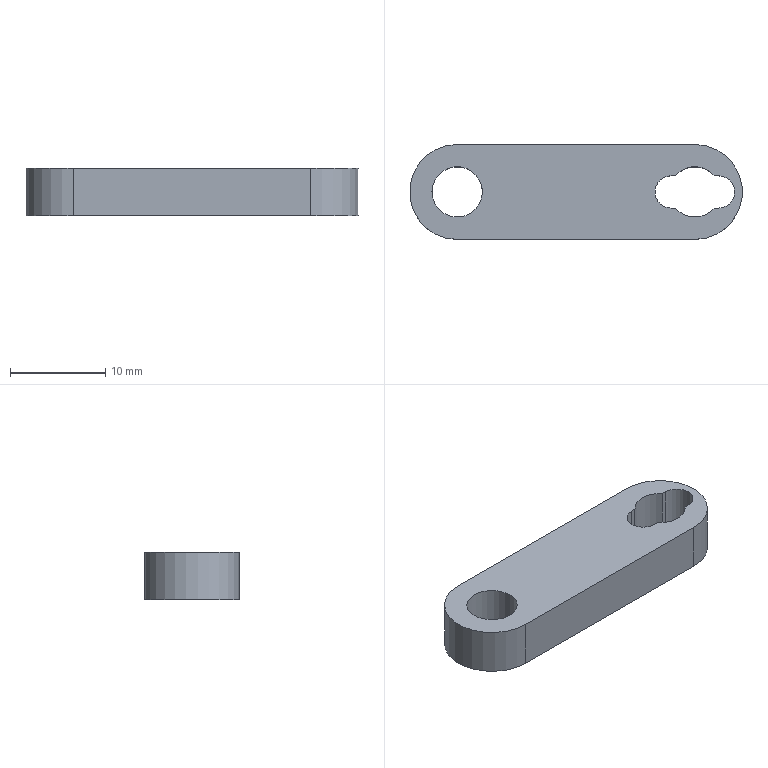Part | NX | features BREP 1 | 1 solid | 15 faces | box 35 x 10 x 5 mm | volume 1375 mm3 | plane 8 | cylinder 7 | commonest cylinder face diameters 5.3 x3 3.4 x2 10 x2
STEP:
#1=CARTESIAN_POINT('',(15.,-1.7,-2.5));
#2=VERTEX_POINT('',#1);
#3=CARTESIAN_POINT('',(15.,1.7,-2.5));
#4=VERTEX_POINT('',#3);
#5=CARTESIAN_POINT('',(15.,0.,-2.5));
#6=DIRECTION('',(0.,0.,1.));
#7=DIRECTION('',(1.,0.,0.));
#8=AXIS2_PLACEMENT_3D('',#5,#6,#7);
#9=CIRCLE('',#8,1.7);
#10=EDGE_CURVE('',#2,#4,#9,.T.);
#11=ORIENTED_EDGE('',*,*,#10,.F.);
#12=CARTESIAN_POINT('',(15.,-1.7,2.5));
#13=VERTEX_POINT('',#12);
#14=CARTESIAN_POINT('',(15.,-1.7,-2.5));
#15=DIRECTION('',(0.,0.,1.));
#16=VECTOR('',#15,1000.);
#17=LINE('',#14,#16);
#18=EDGE_CURVE('',#2,#13,#17,.T.);
#19=ORIENTED_EDGE('',*,*,#18,.T.);
#20=CARTESIAN_POINT('',(15.,1.7,2.5));
#21=VERTEX_POINT('',#20);
#22=CARTESIAN_POINT('',(15.,0.,2.5));
#23=DIRECTION('',(0.,0.,1.));
#24=DIRECTION('',(1.,0.,0.));
#25=AXIS2_PLACEMENT_3D('',#22,#23,#24);
#26=CIRCLE('',#25,1.7);
#27=EDGE_CURVE('',#13,#21,#26,.T.);
#28=ORIENTED_EDGE('',*,*,#27,.T.);
#29=CARTESIAN_POINT('',(15.,1.7,-2.5));
#30=DIRECTION('',(0.,0.,1.));
#31=VECTOR('',#30,1000.);
#32=LINE('',#29,#31);
#33=EDGE_CURVE('',#4,#21,#32,.T.);
#34=ORIENTED_EDGE('',*,*,#33,.F.);
#35=EDGE_LOOP('',(#11,#19,#28,#34));
#36=FACE_BOUND('',#35,.T.);
#37=CARTESIAN_POINT('',(15.,0.,-2.5));
#38=DIRECTION('',(0.,0.,1.));
#39=DIRECTION('',(-1.,0.,0.));
#40=AXIS2_PLACEMENT_3D('',#37,#38,#39);
#41=CYLINDRICAL_SURFACE('',#40,1.7);
#42=ADVANCED_FACE('',(#36),#41,.F.);
#43=CARTESIAN_POINT('',(-9.85,0.,2.5));
#44=VERTEX_POINT('',#43);
#45=CARTESIAN_POINT('',(-12.5,0.,2.5));
#46=DIRECTION('',(0.,0.,1.));
#47=DIRECTION('',(1.,0.,0.));
#48=AXIS2_PLACEMENT_3D('',#45,#46,#47);
#49=CIRCLE('',#48,2.65);
#50=EDGE_CURVE('',#44,#44,#49,.T.);
#51=ORIENTED_EDGE('',*,*,#50,.T.);
#52=EDGE_LOOP('',(#51));
#53=FACE_BOUND('',#52,.T.);
#54=CARTESIAN_POINT('',(-9.85,0.,-2.5));
#55=VERTEX_POINT('',#54);
#56=CARTESIAN_POINT('',(-12.5,0.,-2.5));
#57=DIRECTION('',(0.,0.,1.));
#58=DIRECTION('',(1.,0.,0.));
#59=AXIS2_PLACEMENT_3D('',#56,#57,#58);
#60=CIRCLE('',#59,2.65);
#61=EDGE_CURVE('',#55,#55,#60,.T.);
#62=ORIENTED_EDGE('',*,*,#61,.F.);
#63=EDGE_LOOP('',(#62));
#64=FACE_BOUND('',#63,.T.);
#65=CARTESIAN_POINT('',(-12.5,0.,-2.5));
#66=DIRECTION('',(0.,0.,1.));
#67=DIRECTION('',(-1.,0.,0.));
#68=AXIS2_PLACEMENT_3D('',#65,#66,#67);
#69=CYLINDRICAL_SURFACE('',#68,2.65);
#70=ADVANCED_FACE('',(#53,#64),#69,.F.);
#71=CARTESIAN_POINT('',(-12.5,5.,2.5));
#72=VERTEX_POINT('',#71);
#73=CARTESIAN_POINT('',(-12.5,-5.,2.5));
#74=VERTEX_POINT('',#73);
#75=CARTESIAN_POINT('',(-12.5,0.,2.5));
#76=DIRECTION('',(0.,0.,1.));
#77=DIRECTION('',(1.,0.,0.));
#78=AXIS2_PLACEMENT_3D('',#75,#76,#77);
#79=CIRCLE('',#78,5.);
#80=EDGE_CURVE('',#72,#74,#79,.T.);
#81=ORIENTED_EDGE('',*,*,#80,.F.);
#82=CARTESIAN_POINT('',(-12.5,5.,-2.5));
#83=VERTEX_POINT('',#82);
#84=CARTESIAN_POINT('',(-12.5,5.,2.5));
#85=DIRECTION('',(0.,0.,-1.));
#86=VECTOR('',#85,1000.);
#87=LINE('',#84,#86);
#88=EDGE_CURVE('',#72,#83,#87,.T.);
#89=ORIENTED_EDGE('',*,*,#88,.T.);
#90=CARTESIAN_POINT('',(-12.5,-5.,-2.5));
#91=VERTEX_POINT('',#90);
#92=CARTESIAN_POINT('',(-12.5,0.,-2.5));
#93=DIRECTION('',(0.,0.,1.));
#94=DIRECTION('',(1.,0.,0.));
#95=AXIS2_PLACEMENT_3D('',#92,#93,#94);
#96=CIRCLE('',#95,5.);
#97=EDGE_CURVE('',#83,#91,#96,.T.);
#98=ORIENTED_EDGE('',*,*,#97,.T.);
#99=CARTESIAN_POINT('',(-12.5,-5.,2.5));
#100=DIRECTION('',(0.,0.,-1.));
#101=VECTOR('',#100,1000.);
#102=LINE('',#99,#101);
#103=EDGE_CURVE('',#74,#91,#102,.T.);
#104=ORIENTED_EDGE('',*,*,#103,.F.);
#105=EDGE_LOOP('',(#81,#89,#98,#104));
#106=FACE_BOUND('',#105,.T.);
#107=CARTESIAN_POINT('',(-12.5,0.,2.5));
#108=DIRECTION('',(0.,0.,-1.));
#109=DIRECTION('',(1.,0.,0.));
#110=AXIS2_PLACEMENT_3D('',#107,#108,#109);
#111=CYLINDRICAL_SURFACE('',#110,5.);
#112=ADVANCED_FACE('',(#106),#111,.T.);
#113=CARTESIAN_POINT('',(14.533,1.7,2.5));
#114=VERTEX_POINT('',#113);
#115=CARTESIAN_POINT('',(10.467,1.7,2.5));
#116=VERTEX_POINT('',#115);
#117=CARTESIAN_POINT('',(12.5,0.,2.5));
#118=DIRECTION('',(0.,0.,1.));
#119=DIRECTION('',(1.,0.,0.));
#120=AXIS2_PLACEMENT_3D('',#117,#118,#119);
#121=CIRCLE('',#120,2.65);
#122=EDGE_CURVE('',#114,#116,#121,.T.);
#123=ORIENTED_EDGE('',*,*,#122,.T.);
#124=CARTESIAN_POINT('',(10.467,1.7,-2.5));
#125=VERTEX_POINT('',#124);
#126=CARTESIAN_POINT('',(10.467,1.7,-2.5));
#127=DIRECTION('',(0.,0.,-1.));
#128=VECTOR('',#127,1000.);
#129=LINE('',#126,#128);
#130=EDGE_CURVE('',#116,#125,#129,.T.);
#131=ORIENTED_EDGE('',*,*,#130,.T.);
#132=CARTESIAN_POINT('',(14.533,1.7,-2.5));
#133=VERTEX_POINT('',#132);
#134=CARTESIAN_POINT('',(12.5,0.,-2.5));
#135=DIRECTION('',(0.,0.,1.));
#136=DIRECTION('',(1.,0.,0.));
#137=AXIS2_PLACEMENT_3D('',#134,#135,#136);
#138=CIRCLE('',#137,2.65);
#139=EDGE_CURVE('',#133,#125,#138,.T.);
#140=ORIENTED_EDGE('',*,*,#139,.F.);
#141=CARTESIAN_POINT('',(14.533,1.7,-2.5));
#142=DIRECTION('',(0.,0.,1.));
#143=VECTOR('',#142,1000.);
#144=LINE('',#141,#143);
#145=EDGE_CURVE('',#133,#114,#144,.T.);
#146=ORIENTED_EDGE('',*,*,#145,.T.);
#147=EDGE_LOOP('',(#123,#131,#140,#146));
#148=FACE_BOUND('',#147,.T.);
#149=CARTESIAN_POINT('',(12.5,0.,-2.5));
#150=DIRECTION('',(0.,0.,1.));
#151=DIRECTION('',(-1.,0.,0.));
#152=AXIS2_PLACEMENT_3D('',#149,#150,#151);
#153=CYLINDRICAL_SURFACE('',#152,2.65);
#154=ADVANCED_FACE('',(#148),#153,.F.);
#155=CARTESIAN_POINT('',(12.5,-5.,-2.5));
#156=VERTEX_POINT('',#155);
#157=CARTESIAN_POINT('',(-12.5,-5.,-2.5));
#158=DIRECTION('',(1.,0.,0.));
#159=VECTOR('',#158,1000.);
#160=LINE('',#157,#159);
#161=EDGE_CURVE('',#91,#156,#160,.T.);
#162=ORIENTED_EDGE('',*,*,#161,.T.);
#163=CARTESIAN_POINT('',(12.5,-5.,2.5));
#164=VERTEX_POINT('',#163);
#165=CARTESIAN_POINT('',(12.5,-5.,2.5));
#166=DIRECTION('',(0.,0.,-1.));
#167=VECTOR('',#166,1000.);
#168=LINE('',#165,#167);
#169=EDGE_CURVE('',#164,#156,#168,.T.);
#170=ORIENTED_EDGE('',*,*,#169,.F.);
#171=CARTESIAN_POINT('',(-12.5,-5.,2.5));
#172=DIRECTION('',(1.,0.,0.));
#173=VECTOR('',#172,1000.);
#174=LINE('',#171,#173);
#175=EDGE_CURVE('',#74,#164,#174,.T.);
#176=ORIENTED_EDGE('',*,*,#175,.F.);
#177=ORIENTED_EDGE('',*,*,#103,.T.);
#178=EDGE_LOOP('',(#162,#170,#176,#177));
#179=FACE_BOUND('',#178,.T.);
#180=CARTESIAN_POINT('',(-12.5,-5.,2.5));
#181=DIRECTION('',(0.,1.,0.));
#182=DIRECTION('',(0.,0.,-1.));
#183=AXIS2_PLACEMENT_3D('',#180,#181,#182);
#184=PLANE('',#183);
#185=ADVANCED_FACE('',(#179),#184,.F.);
#186=CARTESIAN_POINT('',(12.5,5.,-2.5));
#187=VERTEX_POINT('',#186);
#188=CARTESIAN_POINT('',(12.5,0.,-2.5));
#189=DIRECTION('',(0.,0.,1.));
#190=DIRECTION('',(1.,0.,0.));
#191=AXIS2_PLACEMENT_3D('',#188,#189,#190);
#192=CIRCLE('',#191,5.);
#193=EDGE_CURVE('',#156,#187,#192,.T.);
#194=ORIENTED_EDGE('',*,*,#193,.T.);
#195=CARTESIAN_POINT('',(12.5,5.,2.5));
#196=VERTEX_POINT('',#195);
#197=CARTESIAN_POINT('',(12.5,5.,2.5));
#198=DIRECTION('',(0.,0.,-1.));
#199=VECTOR('',#198,1000.);
#200=LINE('',#197,#199);
#201=EDGE_CURVE('',#196,#187,#200,.T.);
#202=ORIENTED_EDGE('',*,*,#201,.F.);
#203=CARTESIAN_POINT('',(12.5,0.,2.5));
#204=DIRECTION('',(0.,0.,1.));
#205=DIRECTION('',(1.,0.,0.));
#206=AXIS2_PLACEMENT_3D('',#203,#204,#205);
#207=CIRCLE('',#206,5.);
#208=EDGE_CURVE('',#164,#196,#207,.T.);
#209=ORIENTED_EDGE('',*,*,#208,.F.);
#210=ORIENTED_EDGE('',*,*,#169,.T.);
#211=EDGE_LOOP('',(#194,#202,#209,#210));
#212=FACE_BOUND('',#211,.T.);
#213=CARTESIAN_POINT('',(12.5,0.,2.5));
#214=DIRECTION('',(0.,0.,-1.));
#215=DIRECTION('',(1.,0.,0.));
#216=AXIS2_PLACEMENT_3D('',#213,#214,#215);
#217=CYLINDRICAL_SURFACE('',#216,5.);
#218=ADVANCED_FACE('',(#212),#217,.T.);
#219=CARTESIAN_POINT('',(-12.5,5.,-2.5));
#220=DIRECTION('',(-1.,0.,0.));
#221=VECTOR('',#220,1000.);
#222=LINE('',#219,#221);
#223=EDGE_CURVE('',#187,#83,#222,.T.);
#224=ORIENTED_EDGE('',*,*,#223,.T.);
#225=ORIENTED_EDGE('',*,*,#88,.F.);
#226=CARTESIAN_POINT('',(-12.5,5.,2.5));
#227=DIRECTION('',(-1.,0.,0.));
#228=VECTOR('',#227,1000.);
#229=LINE('',#226,#228);
#230=EDGE_CURVE('',#196,#72,#229,.T.);
#231=ORIENTED_EDGE('',*,*,#230,.F.);
#232=ORIENTED_EDGE('',*,*,#201,.T.);
#233=EDGE_LOOP('',(#224,#225,#231,#232));
#234=FACE_BOUND('',#233,.T.);
#235=CARTESIAN_POINT('',(-12.5,5.,2.5));
#236=DIRECTION('',(0.,-1.,0.));
#237=DIRECTION('',(-1.,0.,0.));
#238=AXIS2_PLACEMENT_3D('',#235,#236,#237);
#239=PLANE('',#238);
#240=ADVANCED_FACE('',(#234),#239,.F.);
#241=CARTESIAN_POINT('',(10.,1.7,2.5));
#242=VERTEX_POINT('',#241);
#243=CARTESIAN_POINT('',(10.,1.7,2.5));
#244=DIRECTION('',(-1.,0.,0.));
#245=VECTOR('',#244,1000.);
#246=LINE('',#243,#245);
#247=EDGE_CURVE('',#116,#242,#246,.T.);
#248=ORIENTED_EDGE('',*,*,#247,.F.);
#249=ORIENTED_EDGE('',*,*,#122,.F.);
#250=CARTESIAN_POINT('',(10.,1.7,2.5));
#251=DIRECTION('',(-1.,0.,0.));
#252=VECTOR('',#251,1000.);
#253=LINE('',#250,#252);
#254=EDGE_CURVE('',#21,#114,#253,.T.);
#255=ORIENTED_EDGE('',*,*,#254,.F.);
#256=ORIENTED_EDGE('',*,*,#27,.F.);
#257=CARTESIAN_POINT('',(14.533,-1.7,2.5));
#258=VERTEX_POINT('',#257);
#259=CARTESIAN_POINT('',(10.,-1.7,2.5));
#260=DIRECTION('',(1.,0.,0.));
#261=VECTOR('',#260,1000.);
#262=LINE('',#259,#261);
#263=EDGE_CURVE('',#258,#13,#262,.T.);
#264=ORIENTED_EDGE('',*,*,#263,.F.);
#265=CARTESIAN_POINT('',(10.467,-1.7,2.5));
#266=VERTEX_POINT('',#265);
#267=CARTESIAN_POINT('',(12.5,0.,2.5));
#268=DIRECTION('',(0.,0.,1.));
#269=DIRECTION('',(1.,0.,0.));
#270=AXIS2_PLACEMENT_3D('',#267,#268,#269);
#271=CIRCLE('',#270,2.65);
#272=EDGE_CURVE('',#266,#258,#271,.T.);
#273=ORIENTED_EDGE('',*,*,#272,.F.);
#274=CARTESIAN_POINT('',(10.,-1.7,2.5));
#275=VERTEX_POINT('',#274);
#276=CARTESIAN_POINT('',(10.,-1.7,2.5));
#277=DIRECTION('',(1.,0.,0.));
#278=VECTOR('',#277,1000.);
#279=LINE('',#276,#278);
#280=EDGE_CURVE('',#275,#266,#279,.T.);
#281=ORIENTED_EDGE('',*,*,#280,.F.);
#282=CARTESIAN_POINT('',(10.,0.,2.5));
#283=DIRECTION('',(0.,0.,1.));
#284=DIRECTION('',(1.,0.,0.));
#285=AXIS2_PLACEMENT_3D('',#282,#283,#284);
#286=CIRCLE('',#285,1.7);
#287=EDGE_CURVE('',#242,#275,#286,.T.);
#288=ORIENTED_EDGE('',*,*,#287,.F.);
#289=EDGE_LOOP('',(#248,#249,#255,#256,#264,#273,#281,#288));
#290=FACE_BOUND('',#289,.T.);
#291=ORIENTED_EDGE('',*,*,#50,.F.);
#292=EDGE_LOOP('',(#291));
#293=FACE_BOUND('',#292,.T.);
#294=ORIENTED_EDGE('',*,*,#230,.T.);
#295=ORIENTED_EDGE('',*,*,#80,.T.);
#296=ORIENTED_EDGE('',*,*,#175,.T.);
#297=ORIENTED_EDGE('',*,*,#208,.T.);
#298=EDGE_LOOP('',(#294,#295,#296,#297));
#299=FACE_BOUND('',#298,.T.);
#300=CARTESIAN_POINT('',(-12.5,0.,2.5));
#301=DIRECTION('',(0.,0.,1.));
#302=DIRECTION('',(-1.,0.,0.));
#303=AXIS2_PLACEMENT_3D('',#300,#301,#302);
#304=PLANE('',#303);
#305=ADVANCED_FACE('',(#290,#293,#299),#304,.T.);
#306=ORIENTED_EDGE('',*,*,#139,.T.);
#307=CARTESIAN_POINT('',(10.,1.7,-2.5));
#308=VERTEX_POINT('',#307);
#309=CARTESIAN_POINT('',(10.,1.7,-2.5));
#310=DIRECTION('',(-1.,0.,0.));
#311=VECTOR('',#310,1000.);
#312=LINE('',#309,#311);
#313=EDGE_CURVE('',#125,#308,#312,.T.);
#314=ORIENTED_EDGE('',*,*,#313,.T.);
#315=CARTESIAN_POINT('',(10.,-1.7,-2.5));
#316=VERTEX_POINT('',#315);
#317=CARTESIAN_POINT('',(10.,0.,-2.5));
#318=DIRECTION('',(0.,0.,1.));
#319=DIRECTION('',(1.,0.,0.));
#320=AXIS2_PLACEMENT_3D('',#317,#318,#319);
#321=CIRCLE('',#320,1.7);
#322=EDGE_CURVE('',#308,#316,#321,.T.);
#323=ORIENTED_EDGE('',*,*,#322,.T.);
#324=CARTESIAN_POINT('',(10.467,-1.7,-2.5));
#325=VERTEX_POINT('',#324);
#326=CARTESIAN_POINT('',(10.,-1.7,-2.5));
#327=DIRECTION('',(1.,0.,0.));
#328=VECTOR('',#327,1000.);
#329=LINE('',#326,#328);
#330=EDGE_CURVE('',#316,#325,#329,.T.);
#331=ORIENTED_EDGE('',*,*,#330,.T.);
#332=CARTESIAN_POINT('',(14.533,-1.7,-2.5));
#333=VERTEX_POINT('',#332);
#334=CARTESIAN_POINT('',(12.5,0.,-2.5));
#335=DIRECTION('',(0.,0.,1.));
#336=DIRECTION('',(1.,0.,0.));
#337=AXIS2_PLACEMENT_3D('',#334,#335,#336);
#338=CIRCLE('',#337,2.65);
#339=EDGE_CURVE('',#325,#333,#338,.T.);
#340=ORIENTED_EDGE('',*,*,#339,.T.);
#341=CARTESIAN_POINT('',(10.,-1.7,-2.5));
#342=DIRECTION('',(1.,0.,0.));
#343=VECTOR('',#342,1000.);
#344=LINE('',#341,#343);
#345=EDGE_CURVE('',#333,#2,#344,.T.);
#346=ORIENTED_EDGE('',*,*,#345,.T.);
#347=ORIENTED_EDGE('',*,*,#10,.T.);
#348=CARTESIAN_POINT('',(10.,1.7,-2.5));
#349=DIRECTION('',(-1.,0.,0.));
#350=VECTOR('',#349,1000.);
#351=LINE('',#348,#350);
#352=EDGE_CURVE('',#4,#133,#351,.T.);
#353=ORIENTED_EDGE('',*,*,#352,.T.);
#354=EDGE_LOOP('',(#306,#314,#323,#331,#340,#346,#347,#353));
#355=FACE_BOUND('',#354,.T.);
#356=ORIENTED_EDGE('',*,*,#61,.T.);
#357=EDGE_LOOP('',(#356));
#358=FACE_BOUND('',#357,.T.);
#359=ORIENTED_EDGE('',*,*,#97,.F.);
#360=ORIENTED_EDGE('',*,*,#223,.F.);
#361=ORIENTED_EDGE('',*,*,#193,.F.);
#362=ORIENTED_EDGE('',*,*,#161,.F.);
#363=EDGE_LOOP('',(#359,#360,#361,#362));
#364=FACE_BOUND('',#363,.T.);
#365=CARTESIAN_POINT('',(-12.5,0.,-2.5));
#366=DIRECTION('',(0.,0.,1.));
#367=DIRECTION('',(-1.,0.,0.));
#368=AXIS2_PLACEMENT_3D('',#365,#366,#367);
#369=PLANE('',#368);
#370=ADVANCED_FACE('',(#355,#358,#364),#369,.F.);
#371=ORIENTED_EDGE('',*,*,#272,.T.);
#372=CARTESIAN_POINT('',(14.533,-1.7,-2.5));
#373=DIRECTION('',(0.,0.,-1.));
#374=VECTOR('',#373,1000.);
#375=LINE('',#372,#374);
#376=EDGE_CURVE('',#258,#333,#375,.T.);
#377=ORIENTED_EDGE('',*,*,#376,.T.);
#378=ORIENTED_EDGE('',*,*,#339,.F.);
#379=CARTESIAN_POINT('',(10.467,-1.7,-2.5));
#380=DIRECTION('',(0.,0.,1.));
#381=VECTOR('',#380,1000.);
#382=LINE('',#379,#381);
#383=EDGE_CURVE('',#325,#266,#382,.T.);
#384=ORIENTED_EDGE('',*,*,#383,.T.);
#385=EDGE_LOOP('',(#371,#377,#378,#384));
#386=FACE_BOUND('',#385,.T.);
#387=CARTESIAN_POINT('',(12.5,0.,-2.5));
#388=DIRECTION('',(0.,0.,1.));
#389=DIRECTION('',(-1.,0.,0.));
#390=AXIS2_PLACEMENT_3D('',#387,#388,#389);
#391=CYLINDRICAL_SURFACE('',#390,2.65);
#392=ADVANCED_FACE('',(#386),#391,.F.);
#393=ORIENTED_EDGE('',*,*,#330,.F.);
#394=CARTESIAN_POINT('',(10.,-1.7,-2.5));
#395=DIRECTION('',(0.,0.,1.));
#396=VECTOR('',#395,1000.);
#397=LINE('',#394,#396);
#398=EDGE_CURVE('',#316,#275,#397,.T.);
#399=ORIENTED_EDGE('',*,*,#398,.T.);
#400=ORIENTED_EDGE('',*,*,#280,.T.);
#401=ORIENTED_EDGE('',*,*,#383,.F.);
#402=EDGE_LOOP('',(#393,#399,#400,#401));
#403=FACE_BOUND('',#402,.T.);
#404=CARTESIAN_POINT('',(10.,-1.7,-2.5));
#405=DIRECTION('',(0.,-1.,0.));
#406=DIRECTION('',(-1.,0.,0.));
#407=AXIS2_PLACEMENT_3D('',#404,#405,#406);
#408=PLANE('',#407);
#409=ADVANCED_FACE('',(#403),#408,.F.);
#410=ORIENTED_EDGE('',*,*,#247,.T.);
#411=CARTESIAN_POINT('',(10.,1.7,-2.5));
#412=DIRECTION('',(0.,0.,1.));
#413=VECTOR('',#412,1000.);
#414=LINE('',#411,#413);
#415=EDGE_CURVE('',#308,#242,#414,.T.);
#416=ORIENTED_EDGE('',*,*,#415,.F.);
#417=ORIENTED_EDGE('',*,*,#313,.F.);
#418=ORIENTED_EDGE('',*,*,#130,.F.);
#419=EDGE_LOOP('',(#410,#416,#417,#418));
#420=FACE_BOUND('',#419,.T.);
#421=CARTESIAN_POINT('',(10.,1.7,-2.5));
#422=DIRECTION('',(0.,1.,0.));
#423=DIRECTION('',(1.,0.,0.));
#424=AXIS2_PLACEMENT_3D('',#421,#422,#423);
#425=PLANE('',#424);
#426=ADVANCED_FACE('',(#420),#425,.F.);
#427=ORIENTED_EDGE('',*,*,#287,.T.);
#428=ORIENTED_EDGE('',*,*,#398,.F.);
#429=ORIENTED_EDGE('',*,*,#322,.F.);
#430=ORIENTED_EDGE('',*,*,#415,.T.);
#431=EDGE_LOOP('',(#427,#428,#429,#430));
#432=FACE_BOUND('',#431,.T.);
#433=CARTESIAN_POINT('',(10.,0.,-2.5));
#434=DIRECTION('',(0.,0.,1.));
#435=DIRECTION('',(-1.,0.,0.));
#436=AXIS2_PLACEMENT_3D('',#433,#434,#435);
#437=CYLINDRICAL_SURFACE('',#436,1.7);
#438=ADVANCED_FACE('',(#432),#437,.F.);
#439=ORIENTED_EDGE('',*,*,#352,.F.);
#440=ORIENTED_EDGE('',*,*,#33,.T.);
#441=ORIENTED_EDGE('',*,*,#254,.T.);
#442=ORIENTED_EDGE('',*,*,#145,.F.);
#443=EDGE_LOOP('',(#439,#440,#441,#442));
#444=FACE_BOUND('',#443,.T.);
#445=CARTESIAN_POINT('',(10.,1.7,-2.5));
#446=DIRECTION('',(0.,1.,0.));
#447=DIRECTION('',(1.,0.,0.));
#448=AXIS2_PLACEMENT_3D('',#445,#446,#447);
#449=PLANE('',#448);
#450=ADVANCED_FACE('',(#444),#449,.F.);
#451=ORIENTED_EDGE('',*,*,#263,.T.);
#452=ORIENTED_EDGE('',*,*,#18,.F.);
#453=ORIENTED_EDGE('',*,*,#345,.F.);
#454=ORIENTED_EDGE('',*,*,#376,.F.);
#455=EDGE_LOOP('',(#451,#452,#453,#454));
#456=FACE_BOUND('',#455,.T.);
#457=CARTESIAN_POINT('',(10.,-1.7,-2.5));
#458=DIRECTION('',(0.,-1.,0.));
#459=DIRECTION('',(-1.,0.,0.));
#460=AXIS2_PLACEMENT_3D('',#457,#458,#459);
#461=PLANE('',#460);
#462=ADVANCED_FACE('',(#456),#461,.F.);
#463=CLOSED_SHELL('',(#42,#70,#112,#154,#185,#218,#240,#305,#370,#392,#409,#426,#438,#450,#462));
#464=MANIFOLD_SOLID_BREP('',#463);
#465=(LENGTH_UNIT()NAMED_UNIT(*)SI_UNIT(.MILLI.,.METRE.));
#466=UNCERTAINTY_MEASURE_WITH_UNIT(LENGTH_MEASURE(0.00001),#465,'','');
#467=(NAMED_UNIT(*)PLANE_ANGLE_UNIT()SI_UNIT($,.RADIAN.));
#468=(NAMED_UNIT(*)SI_UNIT($,.STERADIAN.)SOLID_ANGLE_UNIT());
#469=(GEOMETRIC_REPRESENTATION_CONTEXT(3)GLOBAL_UNCERTAINTY_ASSIGNED_CONTEXT((#466))GLOBAL_UNIT_ASSIGNED_CONTEXT((#465,#467,#468))REPRESENTATION_CONTEXT('',''));
#470=ADVANCED_BREP_SHAPE_REPRESENTATION('',(#464),#469);